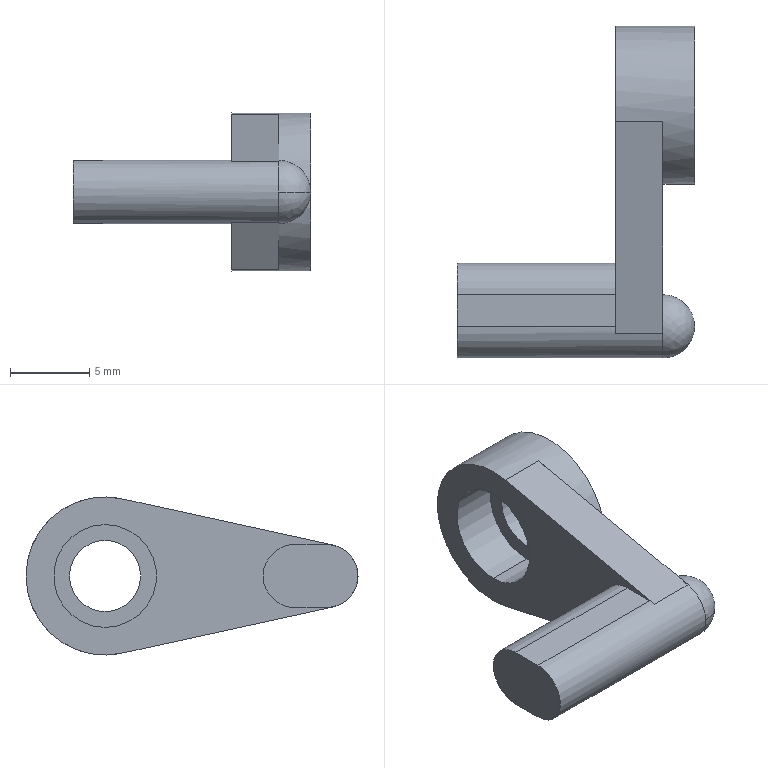Part | STEP file | High-temperature rubber particle | 1 solid | 20 faces | box 15 x 21 x 10 mm | volume 685.576 mm3 | cylinder 9 | plane 9 | spline 2 | commonest cylinder face diameters 4 x3 4.5 x2 6.5 x2 10 x2